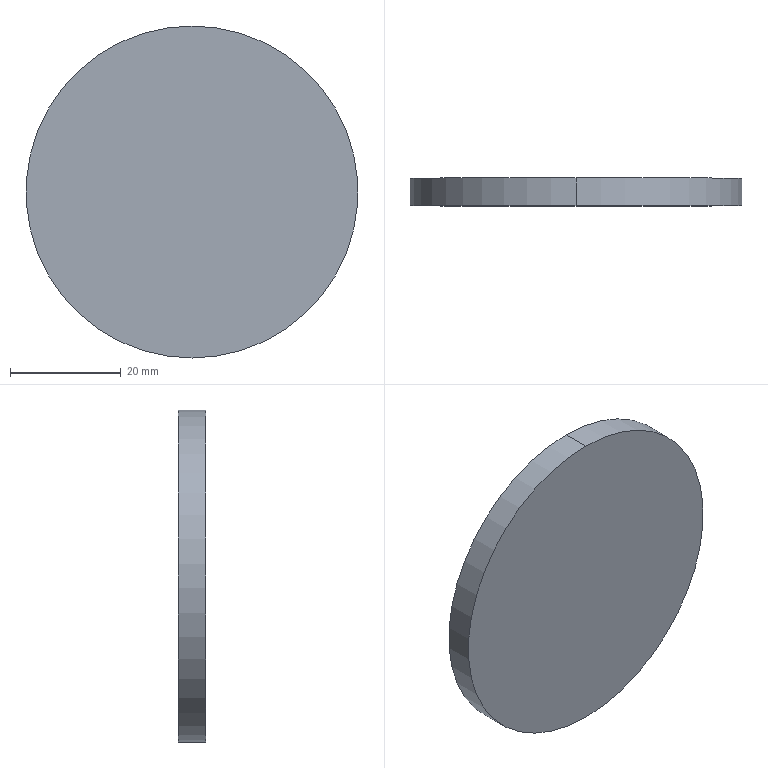Part | SolidWorks | features Extrusion 1 | 1 solid | 4 faces | box 60 x 5 x 60 mm | volume 14137 mm3 | cylinder 2 | plane 2 | commonest cylinder face diameters 60 x2
STEP:
#1=CARTESIAN_POINT('',(0.,5.,30.));
#2=VERTEX_POINT('',#1);
#3=CARTESIAN_POINT('',(0.,5.,-30.));
#4=VERTEX_POINT('',#3);
#5=CARTESIAN_POINT('',(0.,5.,0.));
#6=DIRECTION('',(0.,1.,0.));
#7=DIRECTION('',(0.,0.,1.));
#8=AXIS2_PLACEMENT_3D('',#5,#6,#7);
#9=CIRCLE('',#8,30.);
#10=EDGE_CURVE('',#2,#4,#9,.T.);
#11=ORIENTED_EDGE('',*,*,#10,.F.);
#12=CARTESIAN_POINT('',(0.,0.,30.));
#13=VERTEX_POINT('',#12);
#14=CARTESIAN_POINT('',(0.,5.,30.));
#15=DIRECTION('',(0.,-1.,0.));
#16=VECTOR('',#15,1000.);
#17=LINE('',#14,#16);
#18=EDGE_CURVE('',#2,#13,#17,.T.);
#19=ORIENTED_EDGE('',*,*,#18,.T.);
#20=CARTESIAN_POINT('',(0.,0.,-30.));
#21=VERTEX_POINT('',#20);
#22=CARTESIAN_POINT('',(0.,0.,0.));
#23=DIRECTION('',(0.,1.,0.));
#24=DIRECTION('',(0.,0.,1.));
#25=AXIS2_PLACEMENT_3D('',#22,#23,#24);
#26=CIRCLE('',#25,30.);
#27=EDGE_CURVE('',#13,#21,#26,.T.);
#28=ORIENTED_EDGE('',*,*,#27,.T.);
#29=CARTESIAN_POINT('',(0.,5.,-30.));
#30=DIRECTION('',(0.,-1.,0.));
#31=VECTOR('',#30,1000.);
#32=LINE('',#29,#31);
#33=EDGE_CURVE('',#4,#21,#32,.T.);
#34=ORIENTED_EDGE('',*,*,#33,.F.);
#35=EDGE_LOOP('',(#11,#19,#28,#34));
#36=FACE_OUTER_BOUND('',#35,.T.);
#37=CARTESIAN_POINT('',(0.,5.,0.));
#38=DIRECTION('',(0.,-1.,0.));
#39=DIRECTION('',(0.,0.,-1.));
#40=AXIS2_PLACEMENT_3D('',#37,#38,#39);
#41=CYLINDRICAL_SURFACE('',#40,30.);
#42=ADVANCED_FACE('',(#36),#41,.T.);
#43=ORIENTED_EDGE('',*,*,#18,.F.);
#44=CARTESIAN_POINT('',(0.,5.,0.));
#45=DIRECTION('',(0.,1.,0.));
#46=DIRECTION('',(0.,0.,1.));
#47=AXIS2_PLACEMENT_3D('',#44,#45,#46);
#48=CIRCLE('',#47,30.);
#49=EDGE_CURVE('',#4,#2,#48,.T.);
#50=ORIENTED_EDGE('',*,*,#49,.F.);
#51=ORIENTED_EDGE('',*,*,#33,.T.);
#52=CARTESIAN_POINT('',(0.,0.,0.));
#53=DIRECTION('',(0.,1.,0.));
#54=DIRECTION('',(0.,0.,1.));
#55=AXIS2_PLACEMENT_3D('',#52,#53,#54);
#56=CIRCLE('',#55,30.);
#57=EDGE_CURVE('',#21,#13,#56,.T.);
#58=ORIENTED_EDGE('',*,*,#57,.T.);
#59=EDGE_LOOP('',(#43,#50,#51,#58));
#60=FACE_OUTER_BOUND('',#59,.T.);
#61=CARTESIAN_POINT('',(0.,5.,0.));
#62=DIRECTION('',(0.,-1.,0.));
#63=DIRECTION('',(0.,0.,-1.));
#64=AXIS2_PLACEMENT_3D('',#61,#62,#63);
#65=CYLINDRICAL_SURFACE('',#64,30.);
#66=ADVANCED_FACE('',(#60),#65,.T.);
#67=ORIENTED_EDGE('',*,*,#49,.T.);
#68=ORIENTED_EDGE('',*,*,#10,.T.);
#69=EDGE_LOOP('',(#67,#68));
#70=FACE_OUTER_BOUND('',#69,.T.);
#71=CARTESIAN_POINT('',(0.,5.,0.));
#72=DIRECTION('',(0.,1.,0.));
#73=DIRECTION('',(0.,0.,1.));
#74=AXIS2_PLACEMENT_3D('',#71,#72,#73);
#75=PLANE('',#74);
#76=ADVANCED_FACE('',(#70),#75,.T.);
#77=ORIENTED_EDGE('',*,*,#57,.F.);
#78=ORIENTED_EDGE('',*,*,#27,.F.);
#79=EDGE_LOOP('',(#77,#78));
#80=FACE_OUTER_BOUND('',#79,.T.);
#81=CARTESIAN_POINT('',(0.,0.,0.));
#82=DIRECTION('',(0.,1.,0.));
#83=DIRECTION('',(0.,0.,1.));
#84=AXIS2_PLACEMENT_3D('',#81,#82,#83);
#85=PLANE('',#84);
#86=ADVANCED_FACE('',(#80),#85,.F.);
#87=CLOSED_SHELL('',(#42,#66,#76,#86));
#88=MANIFOLD_SOLID_BREP('',#87);
#89=CARTESIAN_POINT('',(0.,0.,0.));
#90=DIRECTION('',(0.,0.,1.));
#91=DIRECTION('',(1.,0.,0.));
#92=AXIS2_PLACEMENT_3D('',#89,#90,#91);
#93=(LENGTH_UNIT()NAMED_UNIT(*)SI_UNIT(.MILLI.,.METRE.));
#94=UNCERTAINTY_MEASURE_WITH_UNIT(LENGTH_MEASURE(0.00001),#93,'','');
#95=(NAMED_UNIT(*)PLANE_ANGLE_UNIT()SI_UNIT($,.RADIAN.));
#96=(NAMED_UNIT(*)SI_UNIT($,.STERADIAN.)SOLID_ANGLE_UNIT());
#97=(GEOMETRIC_REPRESENTATION_CONTEXT(3)GLOBAL_UNCERTAINTY_ASSIGNED_CONTEXT((#94))GLOBAL_UNIT_ASSIGNED_CONTEXT((#93,#95,#96))REPRESENTATION_CONTEXT('',''));
#98=ADVANCED_BREP_SHAPE_REPRESENTATION('',(#88,#92),#97);